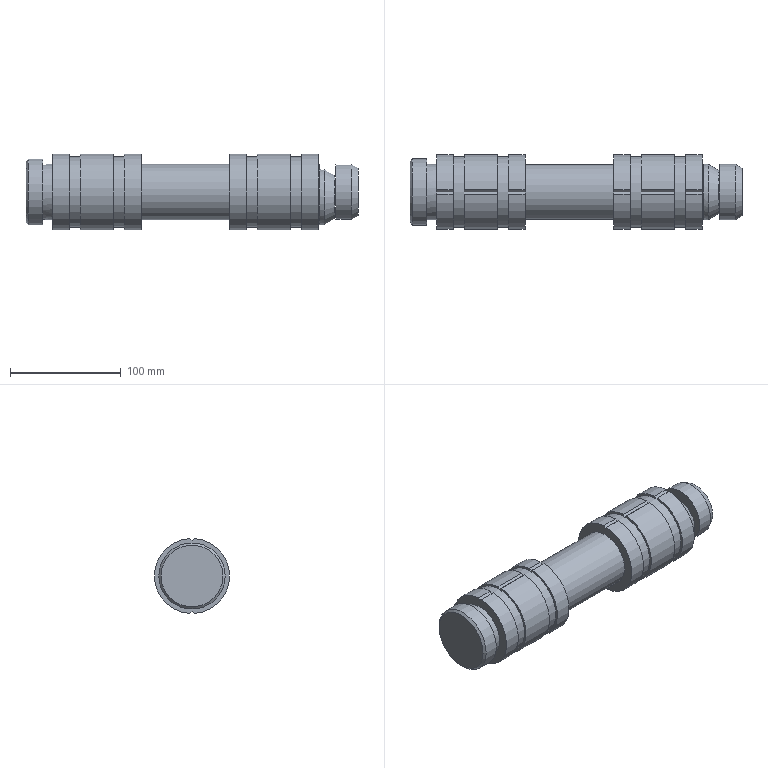Part | NX | features solid 2 | 1 solid | 86 faces | box 300 x 68 x 67.889 mm | volume 837174 mm3 | plane 54 | cylinder 26 | cone 6 | commonest cylinder face diameters 68 x12 50 x5 64 x4 20 x1 20.2 x1 25 x1